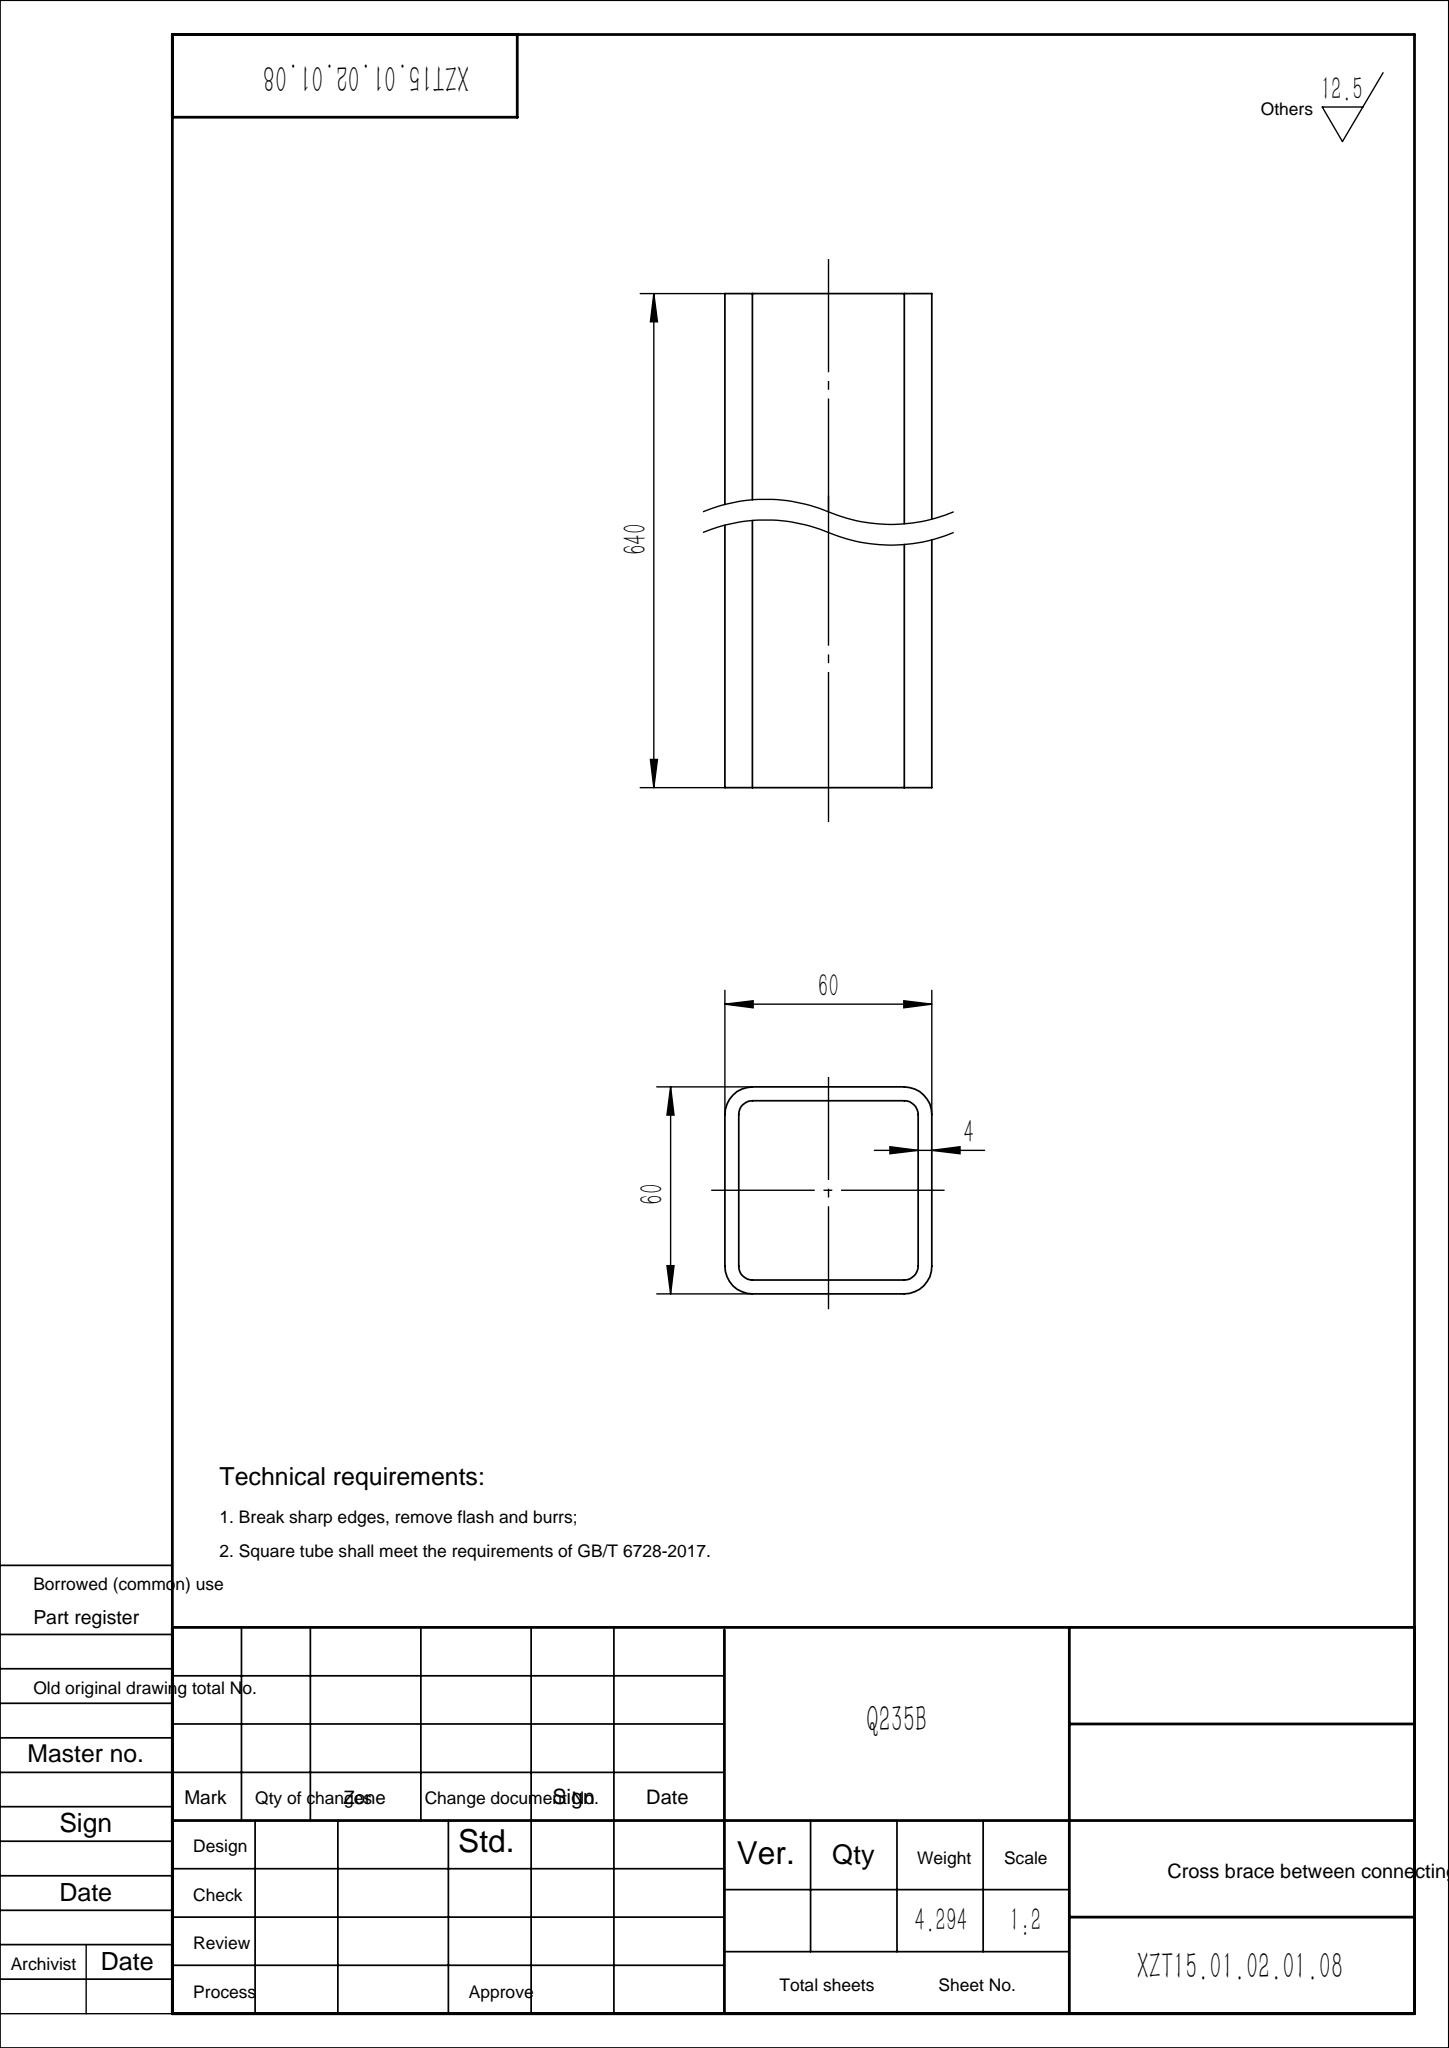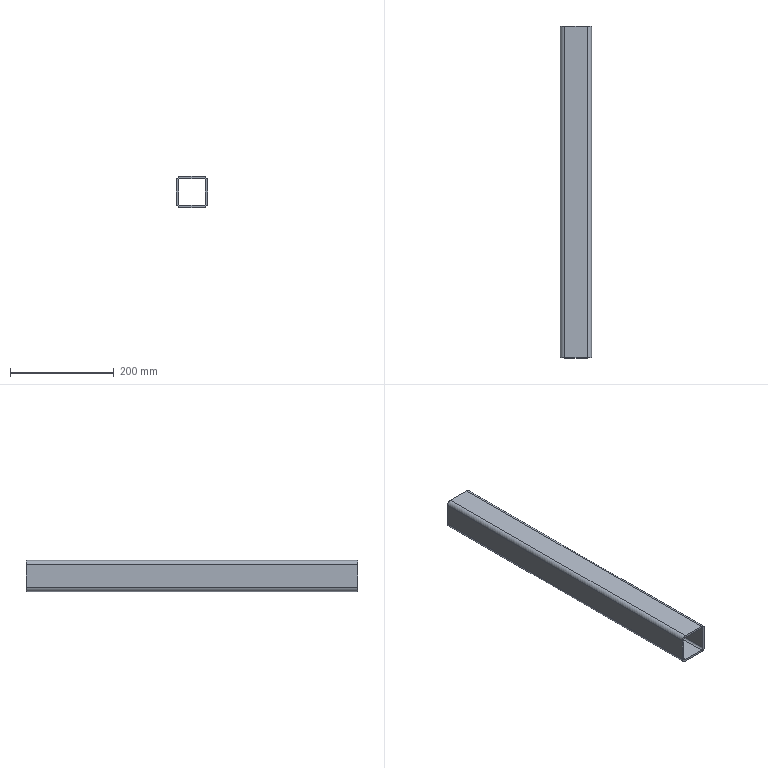Part | SolidWorks | features WeldMemberFeat 1, WeldmentFeature 1 | 1 solid | 18 faces | box 60 x 640 x 60 mm | volume 547070 mm3 | plane 10 | cylinder 8 | commonest cylinder face diameters 8 x4 16 x4
STEP:
#1=CARTESIAN_POINT('',(-30.,0.,22.));
#2=VERTEX_POINT('',#1);
#3=CARTESIAN_POINT('',(-22.,0.,30.));
#4=VERTEX_POINT('',#3);
#5=CARTESIAN_POINT('',(-22.,0.,22.));
#6=DIRECTION('',(0.,1.,0.));
#7=DIRECTION('',(0.,0.,1.));
#8=AXIS2_PLACEMENT_3D('',#5,#6,#7);
#9=CIRCLE('',#8,8.);
#10=EDGE_CURVE('',#2,#4,#9,.T.);
#11=ORIENTED_EDGE('',*,*,#10,.T.);
#12=CARTESIAN_POINT('',(-22.,640.,30.));
#13=VERTEX_POINT('',#12);
#14=CARTESIAN_POINT('',(-22.,640.,30.));
#15=DIRECTION('',(0.,-1.,0.));
#16=VECTOR('',#15,1000.);
#17=LINE('',#14,#16);
#18=EDGE_CURVE('',#13,#4,#17,.T.);
#19=ORIENTED_EDGE('',*,*,#18,.F.);
#20=CARTESIAN_POINT('',(-30.,640.,22.));
#21=VERTEX_POINT('',#20);
#22=CARTESIAN_POINT('',(-22.,640.,22.));
#23=DIRECTION('',(0.,1.,0.));
#24=DIRECTION('',(0.,0.,1.));
#25=AXIS2_PLACEMENT_3D('',#22,#23,#24);
#26=CIRCLE('',#25,8.);
#27=EDGE_CURVE('',#21,#13,#26,.T.);
#28=ORIENTED_EDGE('',*,*,#27,.F.);
#29=CARTESIAN_POINT('',(-30.,640.,22.));
#30=DIRECTION('',(0.,-1.,0.));
#31=VECTOR('',#30,1000.);
#32=LINE('',#29,#31);
#33=EDGE_CURVE('',#21,#2,#32,.T.);
#34=ORIENTED_EDGE('',*,*,#33,.T.);
#35=EDGE_LOOP('',(#11,#19,#28,#34));
#36=FACE_OUTER_BOUND('',#35,.T.);
#37=CARTESIAN_POINT('',(-22.,640.,22.));
#38=DIRECTION('',(0.,-1.,0.));
#39=DIRECTION('',(0.,0.,-1.));
#40=AXIS2_PLACEMENT_3D('',#37,#38,#39);
#41=CYLINDRICAL_SURFACE('',#40,8.);
#42=ADVANCED_FACE('',(#36),#41,.T.);
#43=CARTESIAN_POINT('',(22.,0.,30.));
#44=VERTEX_POINT('',#43);
#45=CARTESIAN_POINT('',(-22.,0.,30.));
#46=DIRECTION('',(1.,0.,0.));
#47=VECTOR('',#46,1000.);
#48=LINE('',#45,#47);
#49=EDGE_CURVE('',#4,#44,#48,.T.);
#50=ORIENTED_EDGE('',*,*,#49,.T.);
#51=CARTESIAN_POINT('',(22.,640.,30.));
#52=VERTEX_POINT('',#51);
#53=CARTESIAN_POINT('',(22.,640.,30.));
#54=DIRECTION('',(0.,-1.,0.));
#55=VECTOR('',#54,1000.);
#56=LINE('',#53,#55);
#57=EDGE_CURVE('',#52,#44,#56,.T.);
#58=ORIENTED_EDGE('',*,*,#57,.F.);
#59=CARTESIAN_POINT('',(-22.,640.,30.));
#60=DIRECTION('',(1.,0.,0.));
#61=VECTOR('',#60,1000.);
#62=LINE('',#59,#61);
#63=EDGE_CURVE('',#13,#52,#62,.T.);
#64=ORIENTED_EDGE('',*,*,#63,.F.);
#65=ORIENTED_EDGE('',*,*,#18,.T.);
#66=EDGE_LOOP('',(#50,#58,#64,#65));
#67=FACE_OUTER_BOUND('',#66,.T.);
#68=CARTESIAN_POINT('',(-22.,640.,30.));
#69=DIRECTION('',(0.,0.,-1.));
#70=DIRECTION('',(-1.,0.,0.));
#71=AXIS2_PLACEMENT_3D('',#68,#69,#70);
#72=PLANE('',#71);
#73=ADVANCED_FACE('',(#67),#72,.F.);
#74=CARTESIAN_POINT('',(30.,0.,22.));
#75=VERTEX_POINT('',#74);
#76=CARTESIAN_POINT('',(22.,0.,22.));
#77=DIRECTION('',(0.,1.,0.));
#78=DIRECTION('',(0.,0.,1.));
#79=AXIS2_PLACEMENT_3D('',#76,#77,#78);
#80=CIRCLE('',#79,8.);
#81=EDGE_CURVE('',#44,#75,#80,.T.);
#82=ORIENTED_EDGE('',*,*,#81,.T.);
#83=CARTESIAN_POINT('',(30.,640.,22.));
#84=VERTEX_POINT('',#83);
#85=CARTESIAN_POINT('',(30.,640.,22.));
#86=DIRECTION('',(0.,-1.,0.));
#87=VECTOR('',#86,1000.);
#88=LINE('',#85,#87);
#89=EDGE_CURVE('',#84,#75,#88,.T.);
#90=ORIENTED_EDGE('',*,*,#89,.F.);
#91=CARTESIAN_POINT('',(22.,640.,22.));
#92=DIRECTION('',(0.,1.,0.));
#93=DIRECTION('',(0.,0.,1.));
#94=AXIS2_PLACEMENT_3D('',#91,#92,#93);
#95=CIRCLE('',#94,8.);
#96=EDGE_CURVE('',#52,#84,#95,.T.);
#97=ORIENTED_EDGE('',*,*,#96,.F.);
#98=ORIENTED_EDGE('',*,*,#57,.T.);
#99=EDGE_LOOP('',(#82,#90,#97,#98));
#100=FACE_OUTER_BOUND('',#99,.T.);
#101=CARTESIAN_POINT('',(22.,640.,22.));
#102=DIRECTION('',(0.,-1.,0.));
#103=DIRECTION('',(0.,0.,-1.));
#104=AXIS2_PLACEMENT_3D('',#101,#102,#103);
#105=CYLINDRICAL_SURFACE('',#104,8.);
#106=ADVANCED_FACE('',(#100),#105,.T.);
#107=CARTESIAN_POINT('',(30.,0.,-22.));
#108=VERTEX_POINT('',#107);
#109=CARTESIAN_POINT('',(30.,0.,-22.));
#110=DIRECTION('',(0.,0.,-1.));
#111=VECTOR('',#110,1000.);
#112=LINE('',#109,#111);
#113=EDGE_CURVE('',#75,#108,#112,.T.);
#114=ORIENTED_EDGE('',*,*,#113,.T.);
#115=CARTESIAN_POINT('',(30.,640.,-22.));
#116=VERTEX_POINT('',#115);
#117=CARTESIAN_POINT('',(30.,640.,-22.));
#118=DIRECTION('',(0.,-1.,0.));
#119=VECTOR('',#118,1000.);
#120=LINE('',#117,#119);
#121=EDGE_CURVE('',#116,#108,#120,.T.);
#122=ORIENTED_EDGE('',*,*,#121,.F.);
#123=CARTESIAN_POINT('',(30.,640.,-22.));
#124=DIRECTION('',(0.,0.,-1.));
#125=VECTOR('',#124,1000.);
#126=LINE('',#123,#125);
#127=EDGE_CURVE('',#84,#116,#126,.T.);
#128=ORIENTED_EDGE('',*,*,#127,.F.);
#129=ORIENTED_EDGE('',*,*,#89,.T.);
#130=EDGE_LOOP('',(#114,#122,#128,#129));
#131=FACE_OUTER_BOUND('',#130,.T.);
#132=CARTESIAN_POINT('',(30.,640.,-22.));
#133=DIRECTION('',(-1.,0.,0.));
#134=DIRECTION('',(0.,0.,1.));
#135=AXIS2_PLACEMENT_3D('',#132,#133,#134);
#136=PLANE('',#135);
#137=ADVANCED_FACE('',(#131),#136,.F.);
#138=CARTESIAN_POINT('',(22.,0.,-30.));
#139=VERTEX_POINT('',#138);
#140=CARTESIAN_POINT('',(22.,0.,-22.));
#141=DIRECTION('',(0.,1.,0.));
#142=DIRECTION('',(0.,0.,1.));
#143=AXIS2_PLACEMENT_3D('',#140,#141,#142);
#144=CIRCLE('',#143,8.);
#145=EDGE_CURVE('',#108,#139,#144,.T.);
#146=ORIENTED_EDGE('',*,*,#145,.T.);
#147=CARTESIAN_POINT('',(22.,640.,-30.));
#148=VERTEX_POINT('',#147);
#149=CARTESIAN_POINT('',(22.,640.,-30.));
#150=DIRECTION('',(0.,-1.,0.));
#151=VECTOR('',#150,1000.);
#152=LINE('',#149,#151);
#153=EDGE_CURVE('',#148,#139,#152,.T.);
#154=ORIENTED_EDGE('',*,*,#153,.F.);
#155=CARTESIAN_POINT('',(22.,640.,-22.));
#156=DIRECTION('',(0.,1.,0.));
#157=DIRECTION('',(0.,0.,1.));
#158=AXIS2_PLACEMENT_3D('',#155,#156,#157);
#159=CIRCLE('',#158,8.);
#160=EDGE_CURVE('',#116,#148,#159,.T.);
#161=ORIENTED_EDGE('',*,*,#160,.F.);
#162=ORIENTED_EDGE('',*,*,#121,.T.);
#163=EDGE_LOOP('',(#146,#154,#161,#162));
#164=FACE_OUTER_BOUND('',#163,.T.);
#165=CARTESIAN_POINT('',(22.,640.,-22.));
#166=DIRECTION('',(0.,-1.,0.));
#167=DIRECTION('',(0.,0.,-1.));
#168=AXIS2_PLACEMENT_3D('',#165,#166,#167);
#169=CYLINDRICAL_SURFACE('',#168,8.);
#170=ADVANCED_FACE('',(#164),#169,.T.);
#171=CARTESIAN_POINT('',(-22.,0.,-30.));
#172=VERTEX_POINT('',#171);
#173=CARTESIAN_POINT('',(22.,0.,-30.));
#174=DIRECTION('',(-1.,0.,0.));
#175=VECTOR('',#174,1000.);
#176=LINE('',#173,#175);
#177=EDGE_CURVE('',#139,#172,#176,.T.);
#178=ORIENTED_EDGE('',*,*,#177,.T.);
#179=CARTESIAN_POINT('',(-22.,640.,-30.));
#180=VERTEX_POINT('',#179);
#181=CARTESIAN_POINT('',(-22.,640.,-30.));
#182=DIRECTION('',(0.,-1.,0.));
#183=VECTOR('',#182,1000.);
#184=LINE('',#181,#183);
#185=EDGE_CURVE('',#180,#172,#184,.T.);
#186=ORIENTED_EDGE('',*,*,#185,.F.);
#187=CARTESIAN_POINT('',(22.,640.,-30.));
#188=DIRECTION('',(-1.,0.,0.));
#189=VECTOR('',#188,1000.);
#190=LINE('',#187,#189);
#191=EDGE_CURVE('',#148,#180,#190,.T.);
#192=ORIENTED_EDGE('',*,*,#191,.F.);
#193=ORIENTED_EDGE('',*,*,#153,.T.);
#194=EDGE_LOOP('',(#178,#186,#192,#193));
#195=FACE_OUTER_BOUND('',#194,.T.);
#196=CARTESIAN_POINT('',(22.,640.,-30.));
#197=DIRECTION('',(0.,0.,1.));
#198=DIRECTION('',(1.,0.,0.));
#199=AXIS2_PLACEMENT_3D('',#196,#197,#198);
#200=PLANE('',#199);
#201=ADVANCED_FACE('',(#195),#200,.F.);
#202=CARTESIAN_POINT('',(-30.,0.,-22.));
#203=VERTEX_POINT('',#202);
#204=CARTESIAN_POINT('',(-22.,0.,-22.));
#205=DIRECTION('',(0.,1.,0.));
#206=DIRECTION('',(0.,0.,1.));
#207=AXIS2_PLACEMENT_3D('',#204,#205,#206);
#208=CIRCLE('',#207,8.);
#209=EDGE_CURVE('',#172,#203,#208,.T.);
#210=ORIENTED_EDGE('',*,*,#209,.T.);
#211=CARTESIAN_POINT('',(-30.,640.,-22.));
#212=VERTEX_POINT('',#211);
#213=CARTESIAN_POINT('',(-30.,640.,-22.));
#214=DIRECTION('',(0.,-1.,0.));
#215=VECTOR('',#214,1000.);
#216=LINE('',#213,#215);
#217=EDGE_CURVE('',#212,#203,#216,.T.);
#218=ORIENTED_EDGE('',*,*,#217,.F.);
#219=CARTESIAN_POINT('',(-22.,640.,-22.));
#220=DIRECTION('',(0.,1.,0.));
#221=DIRECTION('',(0.,0.,1.));
#222=AXIS2_PLACEMENT_3D('',#219,#220,#221);
#223=CIRCLE('',#222,8.);
#224=EDGE_CURVE('',#180,#212,#223,.T.);
#225=ORIENTED_EDGE('',*,*,#224,.F.);
#226=ORIENTED_EDGE('',*,*,#185,.T.);
#227=EDGE_LOOP('',(#210,#218,#225,#226));
#228=FACE_OUTER_BOUND('',#227,.T.);
#229=CARTESIAN_POINT('',(-22.,640.,-22.));
#230=DIRECTION('',(0.,-1.,0.));
#231=DIRECTION('',(0.,0.,-1.));
#232=AXIS2_PLACEMENT_3D('',#229,#230,#231);
#233=CYLINDRICAL_SURFACE('',#232,8.);
#234=ADVANCED_FACE('',(#228),#233,.T.);
#235=CARTESIAN_POINT('',(22.,0.,26.));
#236=VERTEX_POINT('',#235);
#237=CARTESIAN_POINT('',(26.,0.,22.));
#238=VERTEX_POINT('',#237);
#239=CARTESIAN_POINT('',(22.,0.,22.));
#240=DIRECTION('',(0.,1.,0.));
#241=DIRECTION('',(0.,0.,1.));
#242=AXIS2_PLACEMENT_3D('',#239,#240,#241);
#243=CIRCLE('',#242,4.);
#244=EDGE_CURVE('',#236,#238,#243,.T.);
#245=ORIENTED_EDGE('',*,*,#244,.F.);
#246=CARTESIAN_POINT('',(22.,640.,26.));
#247=VERTEX_POINT('',#246);
#248=CARTESIAN_POINT('',(22.,640.,26.));
#249=DIRECTION('',(0.,-1.,0.));
#250=VECTOR('',#249,1000.);
#251=LINE('',#248,#250);
#252=EDGE_CURVE('',#247,#236,#251,.T.);
#253=ORIENTED_EDGE('',*,*,#252,.F.);
#254=CARTESIAN_POINT('',(26.,640.,22.));
#255=VERTEX_POINT('',#254);
#256=CARTESIAN_POINT('',(22.,640.,22.));
#257=DIRECTION('',(0.,1.,0.));
#258=DIRECTION('',(0.,0.,1.));
#259=AXIS2_PLACEMENT_3D('',#256,#257,#258);
#260=CIRCLE('',#259,4.);
#261=EDGE_CURVE('',#247,#255,#260,.T.);
#262=ORIENTED_EDGE('',*,*,#261,.T.);
#263=CARTESIAN_POINT('',(26.,640.,22.));
#264=DIRECTION('',(0.,-1.,0.));
#265=VECTOR('',#264,1000.);
#266=LINE('',#263,#265);
#267=EDGE_CURVE('',#255,#238,#266,.T.);
#268=ORIENTED_EDGE('',*,*,#267,.T.);
#269=EDGE_LOOP('',(#245,#253,#262,#268));
#270=FACE_OUTER_BOUND('',#269,.T.);
#271=CARTESIAN_POINT('',(22.,640.,22.));
#272=DIRECTION('',(0.,-1.,0.));
#273=DIRECTION('',(0.,0.,-1.));
#274=AXIS2_PLACEMENT_3D('',#271,#272,#273);
#275=CYLINDRICAL_SURFACE('',#274,4.);
#276=ADVANCED_FACE('',(#270),#275,.F.);
#277=CARTESIAN_POINT('',(-22.,0.,26.));
#278=VERTEX_POINT('',#277);
#279=CARTESIAN_POINT('',(-22.,0.,26.));
#280=DIRECTION('',(1.,0.,0.));
#281=VECTOR('',#280,1000.);
#282=LINE('',#279,#281);
#283=EDGE_CURVE('',#278,#236,#282,.T.);
#284=ORIENTED_EDGE('',*,*,#283,.F.);
#285=CARTESIAN_POINT('',(-22.,640.,26.));
#286=VERTEX_POINT('',#285);
#287=CARTESIAN_POINT('',(-22.,640.,26.));
#288=DIRECTION('',(0.,-1.,0.));
#289=VECTOR('',#288,1000.);
#290=LINE('',#287,#289);
#291=EDGE_CURVE('',#286,#278,#290,.T.);
#292=ORIENTED_EDGE('',*,*,#291,.F.);
#293=CARTESIAN_POINT('',(-22.,640.,26.));
#294=DIRECTION('',(1.,0.,0.));
#295=VECTOR('',#294,1000.);
#296=LINE('',#293,#295);
#297=EDGE_CURVE('',#286,#247,#296,.T.);
#298=ORIENTED_EDGE('',*,*,#297,.T.);
#299=ORIENTED_EDGE('',*,*,#252,.T.);
#300=EDGE_LOOP('',(#284,#292,#298,#299));
#301=FACE_OUTER_BOUND('',#300,.T.);
#302=CARTESIAN_POINT('',(-22.,640.,26.));
#303=DIRECTION('',(0.,0.,-1.));
#304=DIRECTION('',(-1.,0.,0.));
#305=AXIS2_PLACEMENT_3D('',#302,#303,#304);
#306=PLANE('',#305);
#307=ADVANCED_FACE('',(#301),#306,.T.);
#308=CARTESIAN_POINT('',(-26.,0.,22.));
#309=VERTEX_POINT('',#308);
#310=CARTESIAN_POINT('',(-22.,0.,22.));
#311=DIRECTION('',(0.,1.,0.));
#312=DIRECTION('',(0.,0.,1.));
#313=AXIS2_PLACEMENT_3D('',#310,#311,#312);
#314=CIRCLE('',#313,4.);
#315=EDGE_CURVE('',#309,#278,#314,.T.);
#316=ORIENTED_EDGE('',*,*,#315,.F.);
#317=CARTESIAN_POINT('',(-26.,640.,22.));
#318=VERTEX_POINT('',#317);
#319=CARTESIAN_POINT('',(-26.,640.,22.));
#320=DIRECTION('',(0.,-1.,0.));
#321=VECTOR('',#320,1000.);
#322=LINE('',#319,#321);
#323=EDGE_CURVE('',#318,#309,#322,.T.);
#324=ORIENTED_EDGE('',*,*,#323,.F.);
#325=CARTESIAN_POINT('',(-22.,640.,22.));
#326=DIRECTION('',(0.,1.,0.));
#327=DIRECTION('',(0.,0.,1.));
#328=AXIS2_PLACEMENT_3D('',#325,#326,#327);
#329=CIRCLE('',#328,4.);
#330=EDGE_CURVE('',#318,#286,#329,.T.);
#331=ORIENTED_EDGE('',*,*,#330,.T.);
#332=ORIENTED_EDGE('',*,*,#291,.T.);
#333=EDGE_LOOP('',(#316,#324,#331,#332));
#334=FACE_OUTER_BOUND('',#333,.T.);
#335=CARTESIAN_POINT('',(-22.,640.,22.));
#336=DIRECTION('',(0.,-1.,0.));
#337=DIRECTION('',(0.,0.,-1.));
#338=AXIS2_PLACEMENT_3D('',#335,#336,#337);
#339=CYLINDRICAL_SURFACE('',#338,4.);
#340=ADVANCED_FACE('',(#334),#339,.F.);
#341=CARTESIAN_POINT('',(-26.,0.,-22.));
#342=VERTEX_POINT('',#341);
#343=CARTESIAN_POINT('',(-26.,0.,22.));
#344=DIRECTION('',(0.,0.,1.));
#345=VECTOR('',#344,1000.);
#346=LINE('',#343,#345);
#347=EDGE_CURVE('',#342,#309,#346,.T.);
#348=ORIENTED_EDGE('',*,*,#347,.F.);
#349=CARTESIAN_POINT('',(-26.,640.,-22.));
#350=VERTEX_POINT('',#349);
#351=CARTESIAN_POINT('',(-26.,640.,-22.));
#352=DIRECTION('',(0.,-1.,0.));
#353=VECTOR('',#352,1000.);
#354=LINE('',#351,#353);
#355=EDGE_CURVE('',#350,#342,#354,.T.);
#356=ORIENTED_EDGE('',*,*,#355,.F.);
#357=CARTESIAN_POINT('',(-26.,640.,22.));
#358=DIRECTION('',(0.,0.,1.));
#359=VECTOR('',#358,1000.);
#360=LINE('',#357,#359);
#361=EDGE_CURVE('',#350,#318,#360,.T.);
#362=ORIENTED_EDGE('',*,*,#361,.T.);
#363=ORIENTED_EDGE('',*,*,#323,.T.);
#364=EDGE_LOOP('',(#348,#356,#362,#363));
#365=FACE_OUTER_BOUND('',#364,.T.);
#366=CARTESIAN_POINT('',(-26.,640.,22.));
#367=DIRECTION('',(1.,0.,0.));
#368=DIRECTION('',(0.,0.,-1.));
#369=AXIS2_PLACEMENT_3D('',#366,#367,#368);
#370=PLANE('',#369);
#371=ADVANCED_FACE('',(#365),#370,.T.);
#372=CARTESIAN_POINT('',(-22.,0.,-26.));
#373=VERTEX_POINT('',#372);
#374=CARTESIAN_POINT('',(-22.,0.,-22.));
#375=DIRECTION('',(0.,1.,0.));
#376=DIRECTION('',(0.,0.,1.));
#377=AXIS2_PLACEMENT_3D('',#374,#375,#376);
#378=CIRCLE('',#377,4.);
#379=EDGE_CURVE('',#373,#342,#378,.T.);
#380=ORIENTED_EDGE('',*,*,#379,.F.);
#381=CARTESIAN_POINT('',(-22.,640.,-26.));
#382=VERTEX_POINT('',#381);
#383=CARTESIAN_POINT('',(-22.,640.,-26.));
#384=DIRECTION('',(0.,-1.,0.));
#385=VECTOR('',#384,1000.);
#386=LINE('',#383,#385);
#387=EDGE_CURVE('',#382,#373,#386,.T.);
#388=ORIENTED_EDGE('',*,*,#387,.F.);
#389=CARTESIAN_POINT('',(-22.,640.,-22.));
#390=DIRECTION('',(0.,1.,0.));
#391=DIRECTION('',(0.,0.,1.));
#392=AXIS2_PLACEMENT_3D('',#389,#390,#391);
#393=CIRCLE('',#392,4.);
#394=EDGE_CURVE('',#382,#350,#393,.T.);
#395=ORIENTED_EDGE('',*,*,#394,.T.);
#396=ORIENTED_EDGE('',*,*,#355,.T.);
#397=EDGE_LOOP('',(#380,#388,#395,#396));
#398=FACE_OUTER_BOUND('',#397,.T.);
#399=CARTESIAN_POINT('',(-22.,640.,-22.));
#400=DIRECTION('',(0.,-1.,0.));
#401=DIRECTION('',(0.,0.,-1.));
#402=AXIS2_PLACEMENT_3D('',#399,#400,#401);
#403=CYLINDRICAL_SURFACE('',#402,4.);
#404=ADVANCED_FACE('',(#398),#403,.F.);
#405=CARTESIAN_POINT('',(22.,0.,-26.));
#406=VERTEX_POINT('',#405);
#407=CARTESIAN_POINT('',(22.,0.,-26.));
#408=DIRECTION('',(-1.,0.,0.));
#409=VECTOR('',#408,1000.);
#410=LINE('',#407,#409);
#411=EDGE_CURVE('',#406,#373,#410,.T.);
#412=ORIENTED_EDGE('',*,*,#411,.F.);
#413=CARTESIAN_POINT('',(22.,640.,-26.));
#414=VERTEX_POINT('',#413);
#415=CARTESIAN_POINT('',(22.,640.,-26.));
#416=DIRECTION('',(0.,-1.,0.));
#417=VECTOR('',#416,1000.);
#418=LINE('',#415,#417);
#419=EDGE_CURVE('',#414,#406,#418,.T.);
#420=ORIENTED_EDGE('',*,*,#419,.F.);
#421=CARTESIAN_POINT('',(22.,640.,-26.));
#422=DIRECTION('',(-1.,0.,0.));
#423=VECTOR('',#422,1000.);
#424=LINE('',#421,#423);
#425=EDGE_CURVE('',#414,#382,#424,.T.);
#426=ORIENTED_EDGE('',*,*,#425,.T.);
#427=ORIENTED_EDGE('',*,*,#387,.T.);
#428=EDGE_LOOP('',(#412,#420,#426,#427));
#429=FACE_OUTER_BOUND('',#428,.T.);
#430=CARTESIAN_POINT('',(22.,640.,-26.));
#431=DIRECTION('',(0.,0.,1.));
#432=DIRECTION('',(1.,0.,0.));
#433=AXIS2_PLACEMENT_3D('',#430,#431,#432);
#434=PLANE('',#433);
#435=ADVANCED_FACE('',(#429),#434,.T.);
#436=CARTESIAN_POINT('',(26.,0.,-22.));
#437=VERTEX_POINT('',#436);
#438=CARTESIAN_POINT('',(22.,0.,-22.));
#439=DIRECTION('',(0.,1.,0.));
#440=DIRECTION('',(0.,0.,1.));
#441=AXIS2_PLACEMENT_3D('',#438,#439,#440);
#442=CIRCLE('',#441,4.);
#443=EDGE_CURVE('',#437,#406,#442,.T.);
#444=ORIENTED_EDGE('',*,*,#443,.F.);
#445=CARTESIAN_POINT('',(26.,640.,-22.));
#446=VERTEX_POINT('',#445);
#447=CARTESIAN_POINT('',(26.,640.,-22.));
#448=DIRECTION('',(0.,-1.,0.));
#449=VECTOR('',#448,1000.);
#450=LINE('',#447,#449);
#451=EDGE_CURVE('',#446,#437,#450,.T.);
#452=ORIENTED_EDGE('',*,*,#451,.F.);
#453=CARTESIAN_POINT('',(22.,640.,-22.));
#454=DIRECTION('',(0.,1.,0.));
#455=DIRECTION('',(0.,0.,1.));
#456=AXIS2_PLACEMENT_3D('',#453,#454,#455);
#457=CIRCLE('',#456,4.);
#458=EDGE_CURVE('',#446,#414,#457,.T.);
#459=ORIENTED_EDGE('',*,*,#458,.T.);
#460=ORIENTED_EDGE('',*,*,#419,.T.);
#461=EDGE_LOOP('',(#444,#452,#459,#460));
#462=FACE_OUTER_BOUND('',#461,.T.);
#463=CARTESIAN_POINT('',(22.,640.,-22.));
#464=DIRECTION('',(0.,-1.,0.));
#465=DIRECTION('',(0.,0.,-1.));
#466=AXIS2_PLACEMENT_3D('',#463,#464,#465);
#467=CYLINDRICAL_SURFACE('',#466,4.);
#468=ADVANCED_FACE('',(#462),#467,.F.);
#469=CARTESIAN_POINT('',(26.,0.,-22.));
#470=DIRECTION('',(0.,0.,-1.));
#471=VECTOR('',#470,1000.);
#472=LINE('',#469,#471);
#473=EDGE_CURVE('',#238,#437,#472,.T.);
#474=ORIENTED_EDGE('',*,*,#473,.F.);
#475=ORIENTED_EDGE('',*,*,#267,.F.);
#476=CARTESIAN_POINT('',(26.,640.,-22.));
#477=DIRECTION('',(0.,0.,-1.));
#478=VECTOR('',#477,1000.);
#479=LINE('',#476,#478);
#480=EDGE_CURVE('',#255,#446,#479,.T.);
#481=ORIENTED_EDGE('',*,*,#480,.T.);
#482=ORIENTED_EDGE('',*,*,#451,.T.);
#483=EDGE_LOOP('',(#474,#475,#481,#482));
#484=FACE_OUTER_BOUND('',#483,.T.);
#485=CARTESIAN_POINT('',(26.,640.,-22.));
#486=DIRECTION('',(-1.,0.,0.));
#487=DIRECTION('',(0.,0.,1.));
#488=AXIS2_PLACEMENT_3D('',#485,#486,#487);
#489=PLANE('',#488);
#490=ADVANCED_FACE('',(#484),#489,.T.);
#491=CARTESIAN_POINT('',(-30.,0.,22.));
#492=DIRECTION('',(0.,0.,1.));
#493=VECTOR('',#492,1000.);
#494=LINE('',#491,#493);
#495=EDGE_CURVE('',#203,#2,#494,.T.);
#496=ORIENTED_EDGE('',*,*,#495,.T.);
#497=ORIENTED_EDGE('',*,*,#33,.F.);
#498=CARTESIAN_POINT('',(-30.,640.,22.));
#499=DIRECTION('',(0.,0.,1.));
#500=VECTOR('',#499,1000.);
#501=LINE('',#498,#500);
#502=EDGE_CURVE('',#212,#21,#501,.T.);
#503=ORIENTED_EDGE('',*,*,#502,.F.);
#504=ORIENTED_EDGE('',*,*,#217,.T.);
#505=EDGE_LOOP('',(#496,#497,#503,#504));
#506=FACE_OUTER_BOUND('',#505,.T.);
#507=CARTESIAN_POINT('',(-30.,640.,22.));
#508=DIRECTION('',(1.,0.,0.));
#509=DIRECTION('',(0.,0.,-1.));
#510=AXIS2_PLACEMENT_3D('',#507,#508,#509);
#511=PLANE('',#510);
#512=ADVANCED_FACE('',(#506),#511,.F.);
#513=ORIENTED_EDGE('',*,*,#261,.F.);
#514=ORIENTED_EDGE('',*,*,#297,.F.);
#515=ORIENTED_EDGE('',*,*,#330,.F.);
#516=ORIENTED_EDGE('',*,*,#361,.F.);
#517=ORIENTED_EDGE('',*,*,#394,.F.);
#518=ORIENTED_EDGE('',*,*,#425,.F.);
#519=ORIENTED_EDGE('',*,*,#458,.F.);
#520=ORIENTED_EDGE('',*,*,#480,.F.);
#521=EDGE_LOOP('',(#513,#514,#515,#516,#517,#518,#519,#520));
#522=FACE_BOUND('',#521,.T.);
#523=ORIENTED_EDGE('',*,*,#27,.T.);
#524=ORIENTED_EDGE('',*,*,#63,.T.);
#525=ORIENTED_EDGE('',*,*,#96,.T.);
#526=ORIENTED_EDGE('',*,*,#127,.T.);
#527=ORIENTED_EDGE('',*,*,#160,.T.);
#528=ORIENTED_EDGE('',*,*,#191,.T.);
#529=ORIENTED_EDGE('',*,*,#224,.T.);
#530=ORIENTED_EDGE('',*,*,#502,.T.);
#531=EDGE_LOOP('',(#523,#524,#525,#526,#527,#528,#529,#530));
#532=FACE_OUTER_BOUND('',#531,.T.);
#533=CARTESIAN_POINT('',(-22.,640.,22.));
#534=DIRECTION('',(0.,1.,0.));
#535=DIRECTION('',(0.,0.,1.));
#536=AXIS2_PLACEMENT_3D('',#533,#534,#535);
#537=PLANE('',#536);
#538=ADVANCED_FACE('',(#522,#532),#537,.T.);
#539=ORIENTED_EDGE('',*,*,#244,.T.);
#540=ORIENTED_EDGE('',*,*,#473,.T.);
#541=ORIENTED_EDGE('',*,*,#443,.T.);
#542=ORIENTED_EDGE('',*,*,#411,.T.);
#543=ORIENTED_EDGE('',*,*,#379,.T.);
#544=ORIENTED_EDGE('',*,*,#347,.T.);
#545=ORIENTED_EDGE('',*,*,#315,.T.);
#546=ORIENTED_EDGE('',*,*,#283,.T.);
#547=EDGE_LOOP('',(#539,#540,#541,#542,#543,#544,#545,#546));
#548=FACE_BOUND('',#547,.T.);
#549=ORIENTED_EDGE('',*,*,#10,.F.);
#550=ORIENTED_EDGE('',*,*,#495,.F.);
#551=ORIENTED_EDGE('',*,*,#209,.F.);
#552=ORIENTED_EDGE('',*,*,#177,.F.);
#553=ORIENTED_EDGE('',*,*,#145,.F.);
#554=ORIENTED_EDGE('',*,*,#113,.F.);
#555=ORIENTED_EDGE('',*,*,#81,.F.);
#556=ORIENTED_EDGE('',*,*,#49,.F.);
#557=EDGE_LOOP('',(#549,#550,#551,#552,#553,#554,#555,#556));
#558=FACE_OUTER_BOUND('',#557,.T.);
#559=CARTESIAN_POINT('',(-22.,0.,22.));
#560=DIRECTION('',(0.,1.,0.));
#561=DIRECTION('',(0.,0.,1.));
#562=AXIS2_PLACEMENT_3D('',#559,#560,#561);
#563=PLANE('',#562);
#564=ADVANCED_FACE('',(#548,#558),#563,.F.);
#565=CLOSED_SHELL('',(#42,#73,#106,#137,#170,#201,#234,#276,#307,#340,#371,#404,#435,#468,#490,#512,#538,#564));
#566=MANIFOLD_SOLID_BREP('',#565);
#567=CARTESIAN_POINT('',(0.,0.,0.));
#568=DIRECTION('',(0.,0.,1.));
#569=DIRECTION('',(1.,0.,0.));
#570=AXIS2_PLACEMENT_3D('',#567,#568,#569);
#571=(LENGTH_UNIT()NAMED_UNIT(*)SI_UNIT(.MILLI.,.METRE.));
#572=UNCERTAINTY_MEASURE_WITH_UNIT(LENGTH_MEASURE(0.00001),#571,'','');
#573=(NAMED_UNIT(*)PLANE_ANGLE_UNIT()SI_UNIT($,.RADIAN.));
#574=(NAMED_UNIT(*)SI_UNIT($,.STERADIAN.)SOLID_ANGLE_UNIT());
#575=(GEOMETRIC_REPRESENTATION_CONTEXT(3)GLOBAL_UNCERTAINTY_ASSIGNED_CONTEXT((#572))GLOBAL_UNIT_ASSIGNED_CONTEXT((#571,#573,#574))REPRESENTATION_CONTEXT('',''));
#576=ADVANCED_BREP_SHAPE_REPRESENTATION('',(#566,#570),#575);